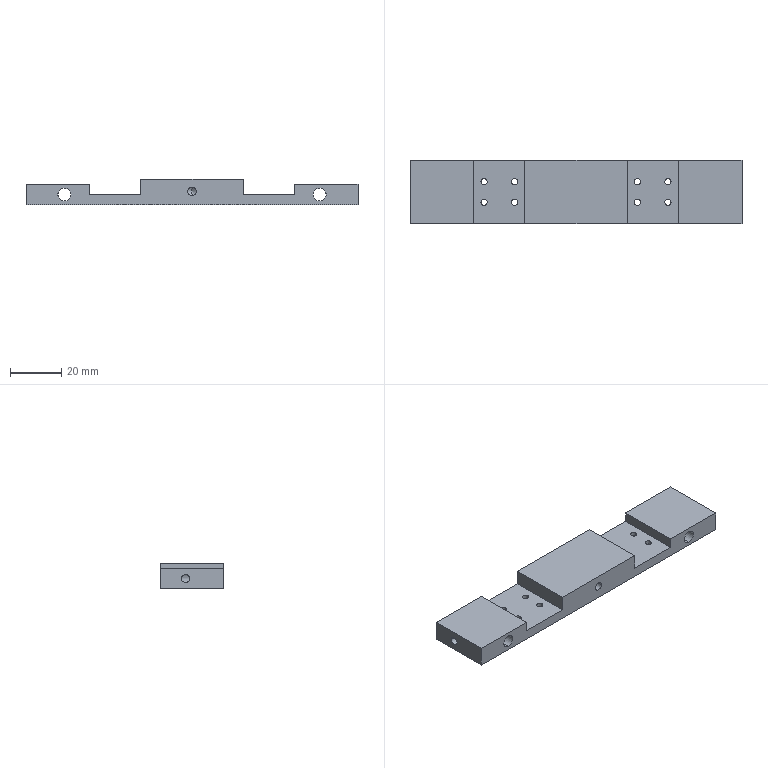Part | SolidWorks | features BaseBody 1 | 1 solid | 66 faces | box 130 x 25 x 10 mm | volume 22368 mm3 | cylinder 42 | plane 22 | cone 2 | commonest cylinder face diameters 2.4 x16 4.5 x16 3.242 x6 5 x4